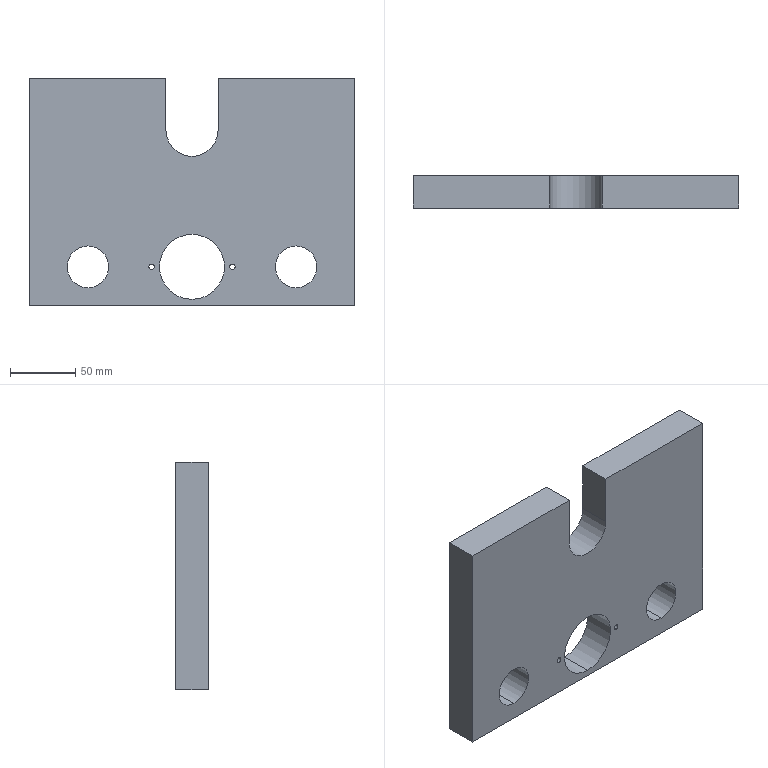Part | SolidWorks | features ICE 3, HoleWzd 2, Extrusion 1, MirrorPattern 1 | 1 solid | 52 faces | box 250 x 25 x 175 mm | volume 946629 mm3 | cylinder 27 | cone 16 | plane 9 | commonest cylinder face diameters 4.2 x20 32 x4 50 x2 40 x1
STEP:
#1=CARTESIAN_POINT('',(-31.,0.,-59.6));
#2=VERTEX_POINT('',#1);
#3=CARTESIAN_POINT('',(-31.,0.,-55.4));
#4=VERTEX_POINT('',#3);
#5=CARTESIAN_POINT('',(-31.,0.,-57.5));
#6=DIRECTION('',(0.,1.,0.));
#7=DIRECTION('',(0.,0.,1.));
#8=AXIS2_PLACEMENT_3D('',#5,#6,#7);
#9=CIRCLE('',#8,2.1);
#10=EDGE_CURVE('',#2,#4,#9,.T.);
#11=ORIENTED_EDGE('',*,*,#10,.F.);
#12=CARTESIAN_POINT('',(-31.,25.,-59.6));
#13=VERTEX_POINT('',#12);
#14=CARTESIAN_POINT('',(-31.,25.,-59.6));
#15=DIRECTION('',(0.,1.,0.));
#16=VECTOR('',#15,1000.);
#17=LINE('',#14,#16);
#18=EDGE_CURVE('',#2,#13,#17,.T.);
#19=ORIENTED_EDGE('',*,*,#18,.T.);
#20=CARTESIAN_POINT('',(-31.,25.,-55.4));
#21=VERTEX_POINT('',#20);
#22=CARTESIAN_POINT('',(-31.,25.,-57.5));
#23=DIRECTION('',(0.,1.,0.));
#24=DIRECTION('',(0.,0.,1.));
#25=AXIS2_PLACEMENT_3D('',#22,#23,#24);
#26=CIRCLE('',#25,2.1);
#27=EDGE_CURVE('',#13,#21,#26,.T.);
#28=ORIENTED_EDGE('',*,*,#27,.T.);
#29=CARTESIAN_POINT('',(-31.,25.,-55.4));
#30=DIRECTION('',(0.,1.,0.));
#31=VECTOR('',#30,1000.);
#32=LINE('',#29,#31);
#33=EDGE_CURVE('',#4,#21,#32,.T.);
#34=ORIENTED_EDGE('',*,*,#33,.F.);
#35=EDGE_LOOP('',(#11,#19,#28,#34));
#36=FACE_OUTER_BOUND('',#35,.T.);
#37=CARTESIAN_POINT('',(-31.,25.,-57.5));
#38=DIRECTION('',(0.,1.,0.));
#39=DIRECTION('',(0.,0.,1.));
#40=AXIS2_PLACEMENT_3D('',#37,#38,#39);
#41=CYLINDRICAL_SURFACE('',#40,2.1);
#42=ADVANCED_FACE('',(#36),#41,.F.);
#43=CARTESIAN_POINT('',(31.,0.,-59.6));
#44=VERTEX_POINT('',#43);
#45=CARTESIAN_POINT('',(31.,0.,-55.4));
#46=VERTEX_POINT('',#45);
#47=CARTESIAN_POINT('',(31.,0.,-57.5));
#48=DIRECTION('',(0.,1.,0.));
#49=DIRECTION('',(0.,0.,1.));
#50=AXIS2_PLACEMENT_3D('',#47,#48,#49);
#51=CIRCLE('',#50,2.1);
#52=EDGE_CURVE('',#44,#46,#51,.T.);
#53=ORIENTED_EDGE('',*,*,#52,.F.);
#54=CARTESIAN_POINT('',(31.,25.,-59.6));
#55=VERTEX_POINT('',#54);
#56=CARTESIAN_POINT('',(31.,25.,-59.6));
#57=DIRECTION('',(0.,1.,0.));
#58=VECTOR('',#57,1000.);
#59=LINE('',#56,#58);
#60=EDGE_CURVE('',#44,#55,#59,.T.);
#61=ORIENTED_EDGE('',*,*,#60,.T.);
#62=CARTESIAN_POINT('',(31.,25.,-55.4));
#63=VERTEX_POINT('',#62);
#64=CARTESIAN_POINT('',(31.,25.,-57.5));
#65=DIRECTION('',(0.,1.,0.));
#66=DIRECTION('',(0.,0.,1.));
#67=AXIS2_PLACEMENT_3D('',#64,#65,#66);
#68=CIRCLE('',#67,2.1);
#69=EDGE_CURVE('',#55,#63,#68,.T.);
#70=ORIENTED_EDGE('',*,*,#69,.T.);
#71=CARTESIAN_POINT('',(31.,25.,-55.4));
#72=DIRECTION('',(0.,1.,0.));
#73=VECTOR('',#72,1000.);
#74=LINE('',#71,#73);
#75=EDGE_CURVE('',#46,#63,#74,.T.);
#76=ORIENTED_EDGE('',*,*,#75,.F.);
#77=EDGE_LOOP('',(#53,#61,#70,#76));
#78=FACE_OUTER_BOUND('',#77,.T.);
#79=CARTESIAN_POINT('',(31.,25.,-57.5));
#80=DIRECTION('',(0.,1.,0.));
#81=DIRECTION('',(0.,0.,1.));
#82=AXIS2_PLACEMENT_3D('',#79,#80,#81);
#83=CYLINDRICAL_SURFACE('',#82,2.1);
#84=ADVANCED_FACE('',(#78),#83,.F.);
#85=CARTESIAN_POINT('',(0.,0.,-82.5));
#86=VERTEX_POINT('',#85);
#87=CARTESIAN_POINT('',(0.,0.,-32.5));
#88=VERTEX_POINT('',#87);
#89=CARTESIAN_POINT('',(0.,0.,-57.5));
#90=DIRECTION('',(0.,1.,0.));
#91=DIRECTION('',(0.,0.,1.));
#92=AXIS2_PLACEMENT_3D('',#89,#90,#91);
#93=CIRCLE('',#92,25.);
#94=EDGE_CURVE('',#86,#88,#93,.T.);
#95=ORIENTED_EDGE('',*,*,#94,.F.);
#96=CARTESIAN_POINT('',(0.,25.,-82.5));
#97=VERTEX_POINT('',#96);
#98=CARTESIAN_POINT('',(0.,0.,-82.5));
#99=DIRECTION('',(0.,1.,0.));
#100=VECTOR('',#99,1000.);
#101=LINE('',#98,#100);
#102=EDGE_CURVE('',#86,#97,#101,.T.);
#103=ORIENTED_EDGE('',*,*,#102,.T.);
#104=CARTESIAN_POINT('',(0.,25.,-32.5));
#105=VERTEX_POINT('',#104);
#106=CARTESIAN_POINT('',(0.,25.,-57.5));
#107=DIRECTION('',(0.,1.,0.));
#108=DIRECTION('',(0.,0.,1.));
#109=AXIS2_PLACEMENT_3D('',#106,#107,#108);
#110=CIRCLE('',#109,25.);
#111=EDGE_CURVE('',#97,#105,#110,.T.);
#112=ORIENTED_EDGE('',*,*,#111,.T.);
#113=CARTESIAN_POINT('',(0.,0.,-32.5));
#114=DIRECTION('',(0.,1.,0.));
#115=VECTOR('',#114,1000.);
#116=LINE('',#113,#115);
#117=EDGE_CURVE('',#88,#105,#116,.T.);
#118=ORIENTED_EDGE('',*,*,#117,.F.);
#119=EDGE_LOOP('',(#95,#103,#112,#118));
#120=FACE_OUTER_BOUND('',#119,.T.);
#121=CARTESIAN_POINT('',(0.,0.,-57.5));
#122=DIRECTION('',(0.,1.,0.));
#123=DIRECTION('',(0.,0.,1.));
#124=AXIS2_PLACEMENT_3D('',#121,#122,#123);
#125=CYLINDRICAL_SURFACE('',#124,25.);
#126=ADVANCED_FACE('',(#120),#125,.F.);
#127=CARTESIAN_POINT('',(92.,12.6,-77.6));
#128=VERTEX_POINT('',#127);
#129=CARTESIAN_POINT('',(92.,12.6,-73.4));
#130=VERTEX_POINT('',#129);
#131=CARTESIAN_POINT('',(92.,12.6,-75.5));
#132=DIRECTION('',(0.,1.,0.));
#133=DIRECTION('',(0.,0.,1.));
#134=AXIS2_PLACEMENT_3D('',#131,#132,#133);
#135=CIRCLE('',#134,2.1);
#136=EDGE_CURVE('',#128,#130,#135,.T.);
#137=ORIENTED_EDGE('',*,*,#136,.F.);
#138=CARTESIAN_POINT('',(92.,25.,-77.6));
#139=VERTEX_POINT('',#138);
#140=CARTESIAN_POINT('',(92.,25.,-77.6));
#141=DIRECTION('',(0.,1.,0.));
#142=VECTOR('',#141,1000.);
#143=LINE('',#140,#142);
#144=EDGE_CURVE('',#128,#139,#143,.T.);
#145=ORIENTED_EDGE('',*,*,#144,.T.);
#146=CARTESIAN_POINT('',(92.,25.,-73.4));
#147=VERTEX_POINT('',#146);
#148=CARTESIAN_POINT('',(92.,25.,-75.5));
#149=DIRECTION('',(0.,1.,0.));
#150=DIRECTION('',(0.,0.,1.));
#151=AXIS2_PLACEMENT_3D('',#148,#149,#150);
#152=CIRCLE('',#151,2.1);
#153=EDGE_CURVE('',#139,#147,#152,.T.);
#154=ORIENTED_EDGE('',*,*,#153,.T.);
#155=CARTESIAN_POINT('',(92.,25.,-73.4));
#156=DIRECTION('',(0.,1.,0.));
#157=VECTOR('',#156,1000.);
#158=LINE('',#155,#157);
#159=EDGE_CURVE('',#130,#147,#158,.T.);
#160=ORIENTED_EDGE('',*,*,#159,.F.);
#161=EDGE_LOOP('',(#137,#145,#154,#160));
#162=FACE_OUTER_BOUND('',#161,.T.);
#163=CARTESIAN_POINT('',(92.,25.,-75.5));
#164=DIRECTION('',(0.,1.,0.));
#165=DIRECTION('',(0.,0.,1.));
#166=AXIS2_PLACEMENT_3D('',#163,#164,#165);
#167=CYLINDRICAL_SURFACE('',#166,2.1);
#168=ADVANCED_FACE('',(#162),#167,.F.);
#169=CARTESIAN_POINT('',(92.,11.338,-75.5));
#170=VERTEX_POINT('',#169);
#171=CARTESIAN_POINT('',(92.,12.6,-73.4));
#172=DIRECTION('',(0.,0.515,0.8572));
#173=VECTOR('',#172,1000.);
#174=LINE('',#171,#173);
#175=EDGE_CURVE('',#170,#130,#174,.T.);
#176=ORIENTED_EDGE('',*,*,#175,.F.);
#177=CARTESIAN_POINT('',(92.,12.6,-77.6));
#178=DIRECTION('',(0.,0.515,-0.8572));
#179=VECTOR('',#178,1000.);
#180=LINE('',#177,#179);
#181=EDGE_CURVE('',#170,#128,#180,.T.);
#182=ORIENTED_EDGE('',*,*,#181,.T.);
#183=ORIENTED_EDGE('',*,*,#136,.T.);
#184=EDGE_LOOP('',(#176,#182,#183));
#185=FACE_OUTER_BOUND('',#184,.T.);
#186=CARTESIAN_POINT('',(92.,12.6,-75.5));
#187=DIRECTION('',(0.,1.,0.));
#188=DIRECTION('',(0.,0.,1.));
#189=AXIS2_PLACEMENT_3D('',#186,#187,#188);
#190=CONICAL_SURFACE('',#189,2.1,1.03);
#191=ADVANCED_FACE('',(#185),#190,.F.);
#192=CARTESIAN_POINT('',(68.,12.6,-77.6));
#193=VERTEX_POINT('',#192);
#194=CARTESIAN_POINT('',(68.,12.6,-73.4));
#195=VERTEX_POINT('',#194);
#196=CARTESIAN_POINT('',(68.,12.6,-75.5));
#197=DIRECTION('',(0.,1.,0.));
#198=DIRECTION('',(0.,0.,1.));
#199=AXIS2_PLACEMENT_3D('',#196,#197,#198);
#200=CIRCLE('',#199,2.1);
#201=EDGE_CURVE('',#193,#195,#200,.T.);
#202=ORIENTED_EDGE('',*,*,#201,.F.);
#203=CARTESIAN_POINT('',(68.,25.,-77.6));
#204=VERTEX_POINT('',#203);
#205=CARTESIAN_POINT('',(68.,25.,-77.6));
#206=DIRECTION('',(0.,1.,0.));
#207=VECTOR('',#206,1000.);
#208=LINE('',#205,#207);
#209=EDGE_CURVE('',#193,#204,#208,.T.);
#210=ORIENTED_EDGE('',*,*,#209,.T.);
#211=CARTESIAN_POINT('',(68.,25.,-73.4));
#212=VERTEX_POINT('',#211);
#213=CARTESIAN_POINT('',(68.,25.,-75.5));
#214=DIRECTION('',(0.,1.,0.));
#215=DIRECTION('',(0.,0.,1.));
#216=AXIS2_PLACEMENT_3D('',#213,#214,#215);
#217=CIRCLE('',#216,2.1);
#218=EDGE_CURVE('',#204,#212,#217,.T.);
#219=ORIENTED_EDGE('',*,*,#218,.T.);
#220=CARTESIAN_POINT('',(68.,25.,-73.4));
#221=DIRECTION('',(0.,1.,0.));
#222=VECTOR('',#221,1000.);
#223=LINE('',#220,#222);
#224=EDGE_CURVE('',#195,#212,#223,.T.);
#225=ORIENTED_EDGE('',*,*,#224,.F.);
#226=EDGE_LOOP('',(#202,#210,#219,#225));
#227=FACE_OUTER_BOUND('',#226,.T.);
#228=CARTESIAN_POINT('',(68.,25.,-75.5));
#229=DIRECTION('',(0.,1.,0.));
#230=DIRECTION('',(0.,0.,1.));
#231=AXIS2_PLACEMENT_3D('',#228,#229,#230);
#232=CYLINDRICAL_SURFACE('',#231,2.1);
#233=ADVANCED_FACE('',(#227),#232,.F.);
#234=CARTESIAN_POINT('',(68.,11.338,-75.5));
#235=VERTEX_POINT('',#234);
#236=CARTESIAN_POINT('',(68.,12.6,-73.4));
#237=DIRECTION('',(0.,0.515,0.8572));
#238=VECTOR('',#237,1000.);
#239=LINE('',#236,#238);
#240=EDGE_CURVE('',#235,#195,#239,.T.);
#241=ORIENTED_EDGE('',*,*,#240,.F.);
#242=CARTESIAN_POINT('',(68.,12.6,-77.6));
#243=DIRECTION('',(0.,0.515,-0.8572));
#244=VECTOR('',#243,1000.);
#245=LINE('',#242,#244);
#246=EDGE_CURVE('',#235,#193,#245,.T.);
#247=ORIENTED_EDGE('',*,*,#246,.T.);
#248=ORIENTED_EDGE('',*,*,#201,.T.);
#249=EDGE_LOOP('',(#241,#247,#248));
#250=FACE_OUTER_BOUND('',#249,.T.);
#251=CARTESIAN_POINT('',(68.,12.6,-75.5));
#252=DIRECTION('',(0.,1.,0.));
#253=DIRECTION('',(0.,0.,1.));
#254=AXIS2_PLACEMENT_3D('',#251,#252,#253);
#255=CONICAL_SURFACE('',#254,2.1,1.03);
#256=ADVANCED_FACE('',(#250),#255,.F.);
#257=CARTESIAN_POINT('',(92.,12.6,-41.6));
#258=VERTEX_POINT('',#257);
#259=CARTESIAN_POINT('',(92.,12.6,-37.4));
#260=VERTEX_POINT('',#259);
#261=CARTESIAN_POINT('',(92.,12.6,-39.5));
#262=DIRECTION('',(0.,1.,0.));
#263=DIRECTION('',(0.,0.,1.));
#264=AXIS2_PLACEMENT_3D('',#261,#262,#263);
#265=CIRCLE('',#264,2.1);
#266=EDGE_CURVE('',#258,#260,#265,.T.);
#267=ORIENTED_EDGE('',*,*,#266,.F.);
#268=CARTESIAN_POINT('',(92.,25.,-41.6));
#269=VERTEX_POINT('',#268);
#270=CARTESIAN_POINT('',(92.,25.,-41.6));
#271=DIRECTION('',(0.,1.,0.));
#272=VECTOR('',#271,1000.);
#273=LINE('',#270,#272);
#274=EDGE_CURVE('',#258,#269,#273,.T.);
#275=ORIENTED_EDGE('',*,*,#274,.T.);
#276=CARTESIAN_POINT('',(92.,25.,-37.4));
#277=VERTEX_POINT('',#276);
#278=CARTESIAN_POINT('',(92.,25.,-39.5));
#279=DIRECTION('',(0.,1.,0.));
#280=DIRECTION('',(0.,0.,1.));
#281=AXIS2_PLACEMENT_3D('',#278,#279,#280);
#282=CIRCLE('',#281,2.1);
#283=EDGE_CURVE('',#269,#277,#282,.T.);
#284=ORIENTED_EDGE('',*,*,#283,.T.);
#285=CARTESIAN_POINT('',(92.,25.,-37.4));
#286=DIRECTION('',(0.,1.,0.));
#287=VECTOR('',#286,1000.);
#288=LINE('',#285,#287);
#289=EDGE_CURVE('',#260,#277,#288,.T.);
#290=ORIENTED_EDGE('',*,*,#289,.F.);
#291=EDGE_LOOP('',(#267,#275,#284,#290));
#292=FACE_OUTER_BOUND('',#291,.T.);
#293=CARTESIAN_POINT('',(92.,25.,-39.5));
#294=DIRECTION('',(0.,1.,0.));
#295=DIRECTION('',(0.,0.,1.));
#296=AXIS2_PLACEMENT_3D('',#293,#294,#295);
#297=CYLINDRICAL_SURFACE('',#296,2.1);
#298=ADVANCED_FACE('',(#292),#297,.F.);
#299=CARTESIAN_POINT('',(92.,11.338,-39.5));
#300=VERTEX_POINT('',#299);
#301=CARTESIAN_POINT('',(92.,12.6,-37.4));
#302=DIRECTION('',(0.,0.515,0.8572));
#303=VECTOR('',#302,1000.);
#304=LINE('',#301,#303);
#305=EDGE_CURVE('',#300,#260,#304,.T.);
#306=ORIENTED_EDGE('',*,*,#305,.F.);
#307=CARTESIAN_POINT('',(92.,12.6,-41.6));
#308=DIRECTION('',(0.,0.515,-0.8572));
#309=VECTOR('',#308,1000.);
#310=LINE('',#307,#309);
#311=EDGE_CURVE('',#300,#258,#310,.T.);
#312=ORIENTED_EDGE('',*,*,#311,.T.);
#313=ORIENTED_EDGE('',*,*,#266,.T.);
#314=EDGE_LOOP('',(#306,#312,#313));
#315=FACE_OUTER_BOUND('',#314,.T.);
#316=CARTESIAN_POINT('',(92.,12.6,-39.5));
#317=DIRECTION('',(0.,1.,0.));
#318=DIRECTION('',(0.,0.,1.));
#319=AXIS2_PLACEMENT_3D('',#316,#317,#318);
#320=CONICAL_SURFACE('',#319,2.1,1.03);
#321=ADVANCED_FACE('',(#315),#320,.F.);
#322=CARTESIAN_POINT('',(68.,12.6,-41.6));
#323=VERTEX_POINT('',#322);
#324=CARTESIAN_POINT('',(68.,12.6,-37.4));
#325=VERTEX_POINT('',#324);
#326=CARTESIAN_POINT('',(68.,12.6,-39.5));
#327=DIRECTION('',(0.,1.,0.));
#328=DIRECTION('',(0.,0.,1.));
#329=AXIS2_PLACEMENT_3D('',#326,#327,#328);
#330=CIRCLE('',#329,2.1);
#331=EDGE_CURVE('',#323,#325,#330,.T.);
#332=ORIENTED_EDGE('',*,*,#331,.F.);
#333=CARTESIAN_POINT('',(68.,25.,-41.6));
#334=VERTEX_POINT('',#333);
#335=CARTESIAN_POINT('',(68.,25.,-41.6));
#336=DIRECTION('',(0.,1.,0.));
#337=VECTOR('',#336,1000.);
#338=LINE('',#335,#337);
#339=EDGE_CURVE('',#323,#334,#338,.T.);
#340=ORIENTED_EDGE('',*,*,#339,.T.);
#341=CARTESIAN_POINT('',(68.,25.,-37.4));
#342=VERTEX_POINT('',#341);
#343=CARTESIAN_POINT('',(68.,25.,-39.5));
#344=DIRECTION('',(0.,1.,0.));
#345=DIRECTION('',(0.,0.,1.));
#346=AXIS2_PLACEMENT_3D('',#343,#344,#345);
#347=CIRCLE('',#346,2.1);
#348=EDGE_CURVE('',#334,#342,#347,.T.);
#349=ORIENTED_EDGE('',*,*,#348,.T.);
#350=CARTESIAN_POINT('',(68.,25.,-37.4));
#351=DIRECTION('',(0.,1.,0.));
#352=VECTOR('',#351,1000.);
#353=LINE('',#350,#352);
#354=EDGE_CURVE('',#325,#342,#353,.T.);
#355=ORIENTED_EDGE('',*,*,#354,.F.);
#356=EDGE_LOOP('',(#332,#340,#349,#355));
#357=FACE_OUTER_BOUND('',#356,.T.);
#358=CARTESIAN_POINT('',(68.,25.,-39.5));
#359=DIRECTION('',(0.,1.,0.));
#360=DIRECTION('',(0.,0.,1.));
#361=AXIS2_PLACEMENT_3D('',#358,#359,#360);
#362=CYLINDRICAL_SURFACE('',#361,2.1);
#363=ADVANCED_FACE('',(#357),#362,.F.);
#364=CARTESIAN_POINT('',(68.,11.338,-39.5));
#365=VERTEX_POINT('',#364);
#366=CARTESIAN_POINT('',(68.,12.6,-37.4));
#367=DIRECTION('',(0.,0.515,0.8572));
#368=VECTOR('',#367,1000.);
#369=LINE('',#366,#368);
#370=EDGE_CURVE('',#365,#325,#369,.T.);
#371=ORIENTED_EDGE('',*,*,#370,.F.);
#372=CARTESIAN_POINT('',(68.,12.6,-41.6));
#373=DIRECTION('',(0.,0.515,-0.8572));
#374=VECTOR('',#373,1000.);
#375=LINE('',#372,#374);
#376=EDGE_CURVE('',#365,#323,#375,.T.);
#377=ORIENTED_EDGE('',*,*,#376,.T.);
#378=ORIENTED_EDGE('',*,*,#331,.T.);
#379=EDGE_LOOP('',(#371,#377,#378));
#380=FACE_OUTER_BOUND('',#379,.T.);
#381=CARTESIAN_POINT('',(68.,12.6,-39.5));
#382=DIRECTION('',(0.,1.,0.));
#383=DIRECTION('',(0.,0.,1.));
#384=AXIS2_PLACEMENT_3D('',#381,#382,#383);
#385=CONICAL_SURFACE('',#384,2.1,1.03);
#386=ADVANCED_FACE('',(#380),#385,.F.);
#387=CARTESIAN_POINT('',(-92.,12.6,-77.6));
#388=VERTEX_POINT('',#387);
#389=CARTESIAN_POINT('',(-92.,12.6,-73.4));
#390=VERTEX_POINT('',#389);
#391=CARTESIAN_POINT('',(-92.,12.6,-75.5));
#392=DIRECTION('',(0.,1.,0.));
#393=DIRECTION('',(0.,0.,1.));
#394=AXIS2_PLACEMENT_3D('',#391,#392,#393);
#395=CIRCLE('',#394,2.1);
#396=EDGE_CURVE('',#388,#390,#395,.T.);
#397=ORIENTED_EDGE('',*,*,#396,.F.);
#398=CARTESIAN_POINT('',(-92.,25.,-77.6));
#399=VERTEX_POINT('',#398);
#400=CARTESIAN_POINT('',(-92.,25.,-77.6));
#401=DIRECTION('',(0.,1.,0.));
#402=VECTOR('',#401,1000.);
#403=LINE('',#400,#402);
#404=EDGE_CURVE('',#388,#399,#403,.T.);
#405=ORIENTED_EDGE('',*,*,#404,.T.);
#406=CARTESIAN_POINT('',(-92.,25.,-73.4));
#407=VERTEX_POINT('',#406);
#408=CARTESIAN_POINT('',(-92.,25.,-75.5));
#409=DIRECTION('',(0.,1.,0.));
#410=DIRECTION('',(0.,0.,1.));
#411=AXIS2_PLACEMENT_3D('',#408,#409,#410);
#412=CIRCLE('',#411,2.1);
#413=EDGE_CURVE('',#399,#407,#412,.T.);
#414=ORIENTED_EDGE('',*,*,#413,.T.);
#415=CARTESIAN_POINT('',(-92.,25.,-73.4));
#416=DIRECTION('',(0.,1.,0.));
#417=VECTOR('',#416,1000.);
#418=LINE('',#415,#417);
#419=EDGE_CURVE('',#390,#407,#418,.T.);
#420=ORIENTED_EDGE('',*,*,#419,.F.);
#421=EDGE_LOOP('',(#397,#405,#414,#420));
#422=FACE_OUTER_BOUND('',#421,.T.);
#423=CARTESIAN_POINT('',(-92.,25.,-75.5));
#424=DIRECTION('',(0.,1.,0.));
#425=DIRECTION('',(0.,0.,1.));
#426=AXIS2_PLACEMENT_3D('',#423,#424,#425);
#427=CYLINDRICAL_SURFACE('',#426,2.1);
#428=ADVANCED_FACE('',(#422),#427,.F.);
#429=CARTESIAN_POINT('',(-92.,11.338,-75.5));
#430=VERTEX_POINT('',#429);
#431=CARTESIAN_POINT('',(-92.,12.6,-73.4));
#432=DIRECTION('',(0.,0.515,0.8572));
#433=VECTOR('',#432,1000.);
#434=LINE('',#431,#433);
#435=EDGE_CURVE('',#430,#390,#434,.T.);
#436=ORIENTED_EDGE('',*,*,#435,.F.);
#437=CARTESIAN_POINT('',(-92.,12.6,-77.6));
#438=DIRECTION('',(0.,0.515,-0.8572));
#439=VECTOR('',#438,1000.);
#440=LINE('',#437,#439);
#441=EDGE_CURVE('',#430,#388,#440,.T.);
#442=ORIENTED_EDGE('',*,*,#441,.T.);
#443=ORIENTED_EDGE('',*,*,#396,.T.);
#444=EDGE_LOOP('',(#436,#442,#443));
#445=FACE_OUTER_BOUND('',#444,.T.);
#446=CARTESIAN_POINT('',(-92.,12.6,-75.5));
#447=DIRECTION('',(0.,1.,0.));
#448=DIRECTION('',(0.,0.,1.));
#449=AXIS2_PLACEMENT_3D('',#446,#447,#448);
#450=CONICAL_SURFACE('',#449,2.1,1.03);
#451=ADVANCED_FACE('',(#445),#450,.F.);
#452=CARTESIAN_POINT('',(-68.,12.6,-77.6));
#453=VERTEX_POINT('',#452);
#454=CARTESIAN_POINT('',(-68.,12.6,-73.4));
#455=VERTEX_POINT('',#454);
#456=CARTESIAN_POINT('',(-68.,12.6,-75.5));
#457=DIRECTION('',(0.,1.,0.));
#458=DIRECTION('',(0.,0.,1.));
#459=AXIS2_PLACEMENT_3D('',#456,#457,#458);
#460=CIRCLE('',#459,2.1);
#461=EDGE_CURVE('',#453,#455,#460,.T.);
#462=ORIENTED_EDGE('',*,*,#461,.F.);
#463=CARTESIAN_POINT('',(-68.,25.,-77.6));
#464=VERTEX_POINT('',#463);
#465=CARTESIAN_POINT('',(-68.,25.,-77.6));
#466=DIRECTION('',(0.,1.,0.));
#467=VECTOR('',#466,1000.);
#468=LINE('',#465,#467);
#469=EDGE_CURVE('',#453,#464,#468,.T.);
#470=ORIENTED_EDGE('',*,*,#469,.T.);
#471=CARTESIAN_POINT('',(-68.,25.,-73.4));
#472=VERTEX_POINT('',#471);
#473=CARTESIAN_POINT('',(-68.,25.,-75.5));
#474=DIRECTION('',(0.,1.,0.));
#475=DIRECTION('',(0.,0.,1.));
#476=AXIS2_PLACEMENT_3D('',#473,#474,#475);
#477=CIRCLE('',#476,2.1);
#478=EDGE_CURVE('',#464,#472,#477,.T.);
#479=ORIENTED_EDGE('',*,*,#478,.T.);
#480=CARTESIAN_POINT('',(-68.,25.,-73.4));
#481=DIRECTION('',(0.,1.,0.));
#482=VECTOR('',#481,1000.);
#483=LINE('',#480,#482);
#484=EDGE_CURVE('',#455,#472,#483,.T.);
#485=ORIENTED_EDGE('',*,*,#484,.F.);
#486=EDGE_LOOP('',(#462,#470,#479,#485));
#487=FACE_OUTER_BOUND('',#486,.T.);
#488=CARTESIAN_POINT('',(-68.,25.,-75.5));
#489=DIRECTION('',(0.,1.,0.));
#490=DIRECTION('',(0.,0.,1.));
#491=AXIS2_PLACEMENT_3D('',#488,#489,#490);
#492=CYLINDRICAL_SURFACE('',#491,2.1);
#493=ADVANCED_FACE('',(#487),#492,.F.);
#494=CARTESIAN_POINT('',(-68.,11.338,-75.5));
#495=VERTEX_POINT('',#494);
#496=CARTESIAN_POINT('',(-68.,12.6,-73.4));
#497=DIRECTION('',(0.,0.515,0.8572));
#498=VECTOR('',#497,1000.);
#499=LINE('',#496,#498);
#500=EDGE_CURVE('',#495,#455,#499,.T.);
#501=ORIENTED_EDGE('',*,*,#500,.F.);
#502=CARTESIAN_POINT('',(-68.,12.6,-77.6));
#503=DIRECTION('',(0.,0.515,-0.8572));
#504=VECTOR('',#503,1000.);
#505=LINE('',#502,#504);
#506=EDGE_CURVE('',#495,#453,#505,.T.);
#507=ORIENTED_EDGE('',*,*,#506,.T.);
#508=ORIENTED_EDGE('',*,*,#461,.T.);
#509=EDGE_LOOP('',(#501,#507,#508));
#510=FACE_OUTER_BOUND('',#509,.T.);
#511=CARTESIAN_POINT('',(-68.,12.6,-75.5));
#512=DIRECTION('',(0.,1.,0.));
#513=DIRECTION('',(0.,0.,1.));
#514=AXIS2_PLACEMENT_3D('',#511,#512,#513);
#515=CONICAL_SURFACE('',#514,2.1,1.03);
#516=ADVANCED_FACE('',(#510),#515,.F.);
#517=CARTESIAN_POINT('',(-92.,12.6,-41.6));
#518=VERTEX_POINT('',#517);
#519=CARTESIAN_POINT('',(-92.,12.6,-37.4));
#520=VERTEX_POINT('',#519);
#521=CARTESIAN_POINT('',(-92.,12.6,-39.5));
#522=DIRECTION('',(0.,1.,0.));
#523=DIRECTION('',(0.,0.,1.));
#524=AXIS2_PLACEMENT_3D('',#521,#522,#523);
#525=CIRCLE('',#524,2.1);
#526=EDGE_CURVE('',#518,#520,#525,.T.);
#527=ORIENTED_EDGE('',*,*,#526,.F.);
#528=CARTESIAN_POINT('',(-92.,25.,-41.6));
#529=VERTEX_POINT('',#528);
#530=CARTESIAN_POINT('',(-92.,25.,-41.6));
#531=DIRECTION('',(0.,1.,0.));
#532=VECTOR('',#531,1000.);
#533=LINE('',#530,#532);
#534=EDGE_CURVE('',#518,#529,#533,.T.);
#535=ORIENTED_EDGE('',*,*,#534,.T.);
#536=CARTESIAN_POINT('',(-92.,25.,-37.4));
#537=VERTEX_POINT('',#536);
#538=CARTESIAN_POINT('',(-92.,25.,-39.5));
#539=DIRECTION('',(0.,1.,0.));
#540=DIRECTION('',(0.,0.,1.));
#541=AXIS2_PLACEMENT_3D('',#538,#539,#540);
#542=CIRCLE('',#541,2.1);
#543=EDGE_CURVE('',#529,#537,#542,.T.);
#544=ORIENTED_EDGE('',*,*,#543,.T.);
#545=CARTESIAN_POINT('',(-92.,25.,-37.4));
#546=DIRECTION('',(0.,1.,0.));
#547=VECTOR('',#546,1000.);
#548=LINE('',#545,#547);
#549=EDGE_CURVE('',#520,#537,#548,.T.);
#550=ORIENTED_EDGE('',*,*,#549,.F.);
#551=EDGE_LOOP('',(#527,#535,#544,#550));
#552=FACE_OUTER_BOUND('',#551,.T.);
#553=CARTESIAN_POINT('',(-92.,25.,-39.5));
#554=DIRECTION('',(0.,1.,0.));
#555=DIRECTION('',(0.,0.,1.));
#556=AXIS2_PLACEMENT_3D('',#553,#554,#555);
#557=CYLINDRICAL_SURFACE('',#556,2.1);
#558=ADVANCED_FACE('',(#552),#557,.F.);
#559=CARTESIAN_POINT('',(-92.,11.338,-39.5));
#560=VERTEX_POINT('',#559);
#561=CARTESIAN_POINT('',(-92.,12.6,-37.4));
#562=DIRECTION('',(0.,0.515,0.8572));
#563=VECTOR('',#562,1000.);
#564=LINE('',#561,#563);
#565=EDGE_CURVE('',#560,#520,#564,.T.);
#566=ORIENTED_EDGE('',*,*,#565,.F.);
#567=CARTESIAN_POINT('',(-92.,12.6,-41.6));
#568=DIRECTION('',(0.,0.515,-0.8572));
#569=VECTOR('',#568,1000.);
#570=LINE('',#567,#569);
#571=EDGE_CURVE('',#560,#518,#570,.T.);
#572=ORIENTED_EDGE('',*,*,#571,.T.);
#573=ORIENTED_EDGE('',*,*,#526,.T.);
#574=EDGE_LOOP('',(#566,#572,#573));
#575=FACE_OUTER_BOUND('',#574,.T.);
#576=CARTESIAN_POINT('',(-92.,12.6,-39.5));
#577=DIRECTION('',(0.,1.,0.));
#578=DIRECTION('',(0.,0.,1.));
#579=AXIS2_PLACEMENT_3D('',#576,#577,#578);
#580=CONICAL_SURFACE('',#579,2.1,1.03);
#581=ADVANCED_FACE('',(#575),#580,.F.);
#582=CARTESIAN_POINT('',(-68.,12.6,-41.6));
#583=VERTEX_POINT('',#582);
#584=CARTESIAN_POINT('',(-68.,12.6,-37.4));
#585=VERTEX_POINT('',#584);
#586=CARTESIAN_POINT('',(-68.,12.6,-39.5));
#587=DIRECTION('',(0.,1.,0.));
#588=DIRECTION('',(0.,0.,1.));
#589=AXIS2_PLACEMENT_3D('',#586,#587,#588);
#590=CIRCLE('',#589,2.1);
#591=EDGE_CURVE('',#583,#585,#590,.T.);
#592=ORIENTED_EDGE('',*,*,#591,.F.);
#593=CARTESIAN_POINT('',(-68.,25.,-41.6));
#594=VERTEX_POINT('',#593);
#595=CARTESIAN_POINT('',(-68.,25.,-41.6));
#596=DIRECTION('',(0.,1.,0.));
#597=VECTOR('',#596,1000.);
#598=LINE('',#595,#597);
#599=EDGE_CURVE('',#583,#594,#598,.T.);
#600=ORIENTED_EDGE('',*,*,#599,.T.);
#601=CARTESIAN_POINT('',(-68.,25.,-37.4));
#602=VERTEX_POINT('',#601);
#603=CARTESIAN_POINT('',(-68.,25.,-39.5));
#604=DIRECTION('',(0.,1.,0.));
#605=DIRECTION('',(0.,0.,1.));
#606=AXIS2_PLACEMENT_3D('',#603,#604,#605);
#607=CIRCLE('',#606,2.1);
#608=EDGE_CURVE('',#594,#602,#607,.T.);
#609=ORIENTED_EDGE('',*,*,#608,.T.);
#610=CARTESIAN_POINT('',(-68.,25.,-37.4));
#611=DIRECTION('',(0.,1.,0.));
#612=VECTOR('',#611,1000.);
#613=LINE('',#610,#612);
#614=EDGE_CURVE('',#585,#602,#613,.T.);
#615=ORIENTED_EDGE('',*,*,#614,.F.);
#616=EDGE_LOOP('',(#592,#600,#609,#615));
#617=FACE_OUTER_BOUND('',#616,.T.);
#618=CARTESIAN_POINT('',(-68.,25.,-39.5));
#619=DIRECTION('',(0.,1.,0.));
#620=DIRECTION('',(0.,0.,1.));
#621=AXIS2_PLACEMENT_3D('',#618,#619,#620);
#622=CYLINDRICAL_SURFACE('',#621,2.1);
#623=ADVANCED_FACE('',(#617),#622,.F.);
#624=CARTESIAN_POINT('',(-68.,11.338,-39.5));
#625=VERTEX_POINT('',#624);
#626=CARTESIAN_POINT('',(-68.,12.6,-37.4));
#627=DIRECTION('',(0.,0.515,0.8572));
#628=VECTOR('',#627,1000.);
#629=LINE('',#626,#628);
#630=EDGE_CURVE('',#625,#585,#629,.T.);
#631=ORIENTED_EDGE('',*,*,#630,.F.);
#632=CARTESIAN_POINT('',(-68.,12.6,-41.6));
#633=DIRECTION('',(0.,0.515,-0.8572));
#634=VECTOR('',#633,1000.);
#635=LINE('',#632,#634);
#636=EDGE_CURVE('',#625,#583,#635,.T.);
#637=ORIENTED_EDGE('',*,*,#636,.T.);
#638=ORIENTED_EDGE('',*,*,#591,.T.);
#639=EDGE_LOOP('',(#631,#637,#638));
#640=FACE_OUTER_BOUND('',#639,.T.);
#641=CARTESIAN_POINT('',(-68.,12.6,-39.5));
#642=DIRECTION('',(0.,1.,0.));
#643=DIRECTION('',(0.,0.,1.));
#644=AXIS2_PLACEMENT_3D('',#641,#642,#643);
#645=CONICAL_SURFACE('',#644,2.1,1.03);
#646=ADVANCED_FACE('',(#640),#645,.F.);
#647=CARTESIAN_POINT('',(-80.,0.,-73.5));
#648=VERTEX_POINT('',#647);
#649=CARTESIAN_POINT('',(-80.,0.,-41.5));
#650=VERTEX_POINT('',#649);
#651=CARTESIAN_POINT('',(-80.,0.,-57.5));
#652=DIRECTION('',(0.,1.,0.));
#653=DIRECTION('',(0.,0.,1.));
#654=AXIS2_PLACEMENT_3D('',#651,#652,#653);
#655=CIRCLE('',#654,16.);
#656=EDGE_CURVE('',#648,#650,#655,.T.);
#657=ORIENTED_EDGE('',*,*,#656,.F.);
#658=CARTESIAN_POINT('',(-80.,25.,-73.5));
#659=VERTEX_POINT('',#658);
#660=CARTESIAN_POINT('',(-80.,0.,-73.5));
#661=DIRECTION('',(0.,1.,0.));
#662=VECTOR('',#661,1000.);
#663=LINE('',#660,#662);
#664=EDGE_CURVE('',#648,#659,#663,.T.);
#665=ORIENTED_EDGE('',*,*,#664,.T.);
#666=CARTESIAN_POINT('',(-80.,25.,-41.5));
#667=VERTEX_POINT('',#666);
#668=CARTESIAN_POINT('',(-80.,25.,-57.5));
#669=DIRECTION('',(0.,1.,0.));
#670=DIRECTION('',(0.,0.,1.));
#671=AXIS2_PLACEMENT_3D('',#668,#669,#670);
#672=CIRCLE('',#671,16.);
#673=EDGE_CURVE('',#659,#667,#672,.T.);
#674=ORIENTED_EDGE('',*,*,#673,.T.);
#675=CARTESIAN_POINT('',(-80.,0.,-41.5));
#676=DIRECTION('',(0.,1.,0.));
#677=VECTOR('',#676,1000.);
#678=LINE('',#675,#677);
#679=EDGE_CURVE('',#650,#667,#678,.T.);
#680=ORIENTED_EDGE('',*,*,#679,.F.);
#681=EDGE_LOOP('',(#657,#665,#674,#680));
#682=FACE_OUTER_BOUND('',#681,.T.);
#683=CARTESIAN_POINT('',(-80.,0.,-57.5));
#684=DIRECTION('',(0.,1.,0.));
#685=DIRECTION('',(0.,0.,1.));
#686=AXIS2_PLACEMENT_3D('',#683,#684,#685);
#687=CYLINDRICAL_SURFACE('',#686,16.);
#688=ADVANCED_FACE('',(#682),#687,.F.);
#689=CARTESIAN_POINT('',(80.,0.,-73.5));
#690=VERTEX_POINT('',#689);
#691=CARTESIAN_POINT('',(80.,0.,-41.5));
#692=VERTEX_POINT('',#691);
#693=CARTESIAN_POINT('',(80.,0.,-57.5));
#694=DIRECTION('',(0.,1.,0.));
#695=DIRECTION('',(0.,0.,-1.));
#696=AXIS2_PLACEMENT_3D('',#693,#694,#695);
#697=CIRCLE('',#696,16.);
#698=EDGE_CURVE('',#690,#692,#697,.T.);
#699=ORIENTED_EDGE('',*,*,#698,.F.);
#700=CARTESIAN_POINT('',(80.,25.,-73.5));
#701=VERTEX_POINT('',#700);
#702=CARTESIAN_POINT('',(80.,0.,-73.5));
#703=DIRECTION('',(0.,1.,0.));
#704=VECTOR('',#703,1000.);
#705=LINE('',#702,#704);
#706=EDGE_CURVE('',#690,#701,#705,.T.);
#707=ORIENTED_EDGE('',*,*,#706,.T.);
#708=CARTESIAN_POINT('',(80.,25.,-41.5));
#709=VERTEX_POINT('',#708);
#710=CARTESIAN_POINT('',(80.,25.,-57.5));
#711=DIRECTION('',(0.,1.,0.));
#712=DIRECTION('',(0.,0.,-1.));
#713=AXIS2_PLACEMENT_3D('',#710,#711,#712);
#714=CIRCLE('',#713,16.);
#715=EDGE_CURVE('',#701,#709,#714,.T.);
#716=ORIENTED_EDGE('',*,*,#715,.T.);
#717=CARTESIAN_POINT('',(80.,0.,-41.5));
#718=DIRECTION('',(0.,1.,0.));
#719=VECTOR('',#718,1000.);
#720=LINE('',#717,#719);
#721=EDGE_CURVE('',#692,#709,#720,.T.);
#722=ORIENTED_EDGE('',*,*,#721,.F.);
#723=EDGE_LOOP('',(#699,#707,#716,#722));
#724=FACE_OUTER_BOUND('',#723,.T.);
#725=CARTESIAN_POINT('',(80.,0.,-57.5));
#726=DIRECTION('',(0.,1.,0.));
#727=DIRECTION('',(0.,0.,1.));
#728=AXIS2_PLACEMENT_3D('',#725,#726,#727);
#729=CYLINDRICAL_SURFACE('',#728,16.);
#730=ADVANCED_FACE('',(#724),#729,.F.);
#731=CARTESIAN_POINT('',(20.,25.,87.5));
#732=VERTEX_POINT('',#731);
#733=CARTESIAN_POINT('',(125.,25.,87.5));
#734=VERTEX_POINT('',#733);
#735=CARTESIAN_POINT('',(-125.,25.,87.5));
#736=DIRECTION('',(1.,0.,0.));
#737=VECTOR('',#736,1000.);
#738=LINE('',#735,#737);
#739=EDGE_CURVE('',#732,#734,#738,.T.);
#740=ORIENTED_EDGE('',*,*,#739,.F.);
#741=CARTESIAN_POINT('',(20.,0.,87.5));
#742=VERTEX_POINT('',#741);
#743=CARTESIAN_POINT('',(20.,0.,87.5));
#744=DIRECTION('',(0.,1.,0.));
#745=VECTOR('',#744,1000.);
#746=LINE('',#743,#745);
#747=EDGE_CURVE('',#742,#732,#746,.T.);
#748=ORIENTED_EDGE('',*,*,#747,.F.);
#749=CARTESIAN_POINT('',(125.,0.,87.5));
#750=VERTEX_POINT('',#749);
#751=CARTESIAN_POINT('',(-125.,0.,87.5));
#752=DIRECTION('',(1.,0.,0.));
#753=VECTOR('',#752,1000.);
#754=LINE('',#751,#753);
#755=EDGE_CURVE('',#742,#750,#754,.T.);
#756=ORIENTED_EDGE('',*,*,#755,.T.);
#757=CARTESIAN_POINT('',(125.,25.,87.5));
#758=DIRECTION('',(0.,-1.,0.));
#759=VECTOR('',#758,1000.);
#760=LINE('',#757,#759);
#761=EDGE_CURVE('',#734,#750,#760,.T.);
#762=ORIENTED_EDGE('',*,*,#761,.F.);
#763=EDGE_LOOP('',(#740,#748,#756,#762));
#764=FACE_OUTER_BOUND('',#763,.T.);
#765=CARTESIAN_POINT('',(-125.,25.,87.5));
#766=DIRECTION('',(0.,0.,-1.));
#767=DIRECTION('',(-1.,0.,0.));
#768=AXIS2_PLACEMENT_3D('',#765,#766,#767);
#769=PLANE('',#768);
#770=ADVANCED_FACE('',(#764),#769,.F.);
#771=CARTESIAN_POINT('',(125.,0.,-87.5));
#772=VERTEX_POINT('',#771);
#773=CARTESIAN_POINT('',(125.,0.,-87.5));
#774=DIRECTION('',(0.,0.,-1.));
#775=VECTOR('',#774,1000.);
#776=LINE('',#773,#775);
#777=EDGE_CURVE('',#750,#772,#776,.T.);
#778=ORIENTED_EDGE('',*,*,#777,.T.);
#779=CARTESIAN_POINT('',(125.,25.,-87.5));
#780=VERTEX_POINT('',#779);
#781=CARTESIAN_POINT('',(125.,25.,-87.5));
#782=DIRECTION('',(0.,-1.,0.));
#783=VECTOR('',#782,1000.);
#784=LINE('',#781,#783);
#785=EDGE_CURVE('',#780,#772,#784,.T.);
#786=ORIENTED_EDGE('',*,*,#785,.F.);
#787=CARTESIAN_POINT('',(125.,25.,-87.5));
#788=DIRECTION('',(0.,0.,-1.));
#789=VECTOR('',#788,1000.);
#790=LINE('',#787,#789);
#791=EDGE_CURVE('',#734,#780,#790,.T.);
#792=ORIENTED_EDGE('',*,*,#791,.F.);
#793=ORIENTED_EDGE('',*,*,#761,.T.);
#794=EDGE_LOOP('',(#778,#786,#792,#793));
#795=FACE_OUTER_BOUND('',#794,.T.);
#796=CARTESIAN_POINT('',(125.,25.,-87.5));
#797=DIRECTION('',(-1.,0.,0.));
#798=DIRECTION('',(0.,0.,1.));
#799=AXIS2_PLACEMENT_3D('',#796,#797,#798);
#800=PLANE('',#799);
#801=ADVANCED_FACE('',(#795),#800,.F.);
#802=CARTESIAN_POINT('',(-125.,0.,-87.5));
#803=VERTEX_POINT('',#802);
#804=CARTESIAN_POINT('',(-125.,0.,-87.5));
#805=DIRECTION('',(-1.,0.,0.));
#806=VECTOR('',#805,1000.);
#807=LINE('',#804,#806);
#808=EDGE_CURVE('',#772,#803,#807,.T.);
#809=ORIENTED_EDGE('',*,*,#808,.T.);
#810=CARTESIAN_POINT('',(-125.,25.,-87.5));
#811=VERTEX_POINT('',#810);
#812=CARTESIAN_POINT('',(-125.,25.,-87.5));
#813=DIRECTION('',(0.,-1.,0.));
#814=VECTOR('',#813,1000.);
#815=LINE('',#812,#814);
#816=EDGE_CURVE('',#811,#803,#815,.T.);
#817=ORIENTED_EDGE('',*,*,#816,.F.);
#818=CARTESIAN_POINT('',(-125.,25.,-87.5));
#819=DIRECTION('',(-1.,0.,0.));
#820=VECTOR('',#819,1000.);
#821=LINE('',#818,#820);
#822=EDGE_CURVE('',#780,#811,#821,.T.);
#823=ORIENTED_EDGE('',*,*,#822,.F.);
#824=ORIENTED_EDGE('',*,*,#785,.T.);
#825=EDGE_LOOP('',(#809,#817,#823,#824));
#826=FACE_OUTER_BOUND('',#825,.T.);
#827=CARTESIAN_POINT('',(-125.,25.,-87.5));
#828=DIRECTION('',(0.,0.,1.));
#829=DIRECTION('',(1.,0.,0.));
#830=AXIS2_PLACEMENT_3D('',#827,#828,#829);
#831=PLANE('',#830);
#832=ADVANCED_FACE('',(#826),#831,.F.);
#833=CARTESIAN_POINT('',(-125.,0.,87.5));
#834=VERTEX_POINT('',#833);
#835=CARTESIAN_POINT('',(-125.,0.,-87.5));
#836=DIRECTION('',(0.,0.,1.));
#837=VECTOR('',#836,1000.);
#838=LINE('',#835,#837);
#839=EDGE_CURVE('',#803,#834,#838,.T.);
#840=ORIENTED_EDGE('',*,*,#839,.T.);
#841=CARTESIAN_POINT('',(-125.,25.,87.5));
#842=VERTEX_POINT('',#841);
#843=CARTESIAN_POINT('',(-125.,25.,87.5));
#844=DIRECTION('',(0.,-1.,0.));
#845=VECTOR('',#844,1000.);
#846=LINE('',#843,#845);
#847=EDGE_CURVE('',#842,#834,#846,.T.);
#848=ORIENTED_EDGE('',*,*,#847,.F.);
#849=CARTESIAN_POINT('',(-125.,25.,-87.5));
#850=DIRECTION('',(0.,0.,1.));
#851=VECTOR('',#850,1000.);
#852=LINE('',#849,#851);
#853=EDGE_CURVE('',#811,#842,#852,.T.);
#854=ORIENTED_EDGE('',*,*,#853,.F.);
#855=ORIENTED_EDGE('',*,*,#816,.T.);
#856=EDGE_LOOP('',(#840,#848,#854,#855));
#857=FACE_OUTER_BOUND('',#856,.T.);
#858=CARTESIAN_POINT('',(-125.,25.,-87.5));
#859=DIRECTION('',(1.,0.,0.));
#860=DIRECTION('',(0.,0.,-1.));
#861=AXIS2_PLACEMENT_3D('',#858,#859,#860);
#862=PLANE('',#861);
#863=ADVANCED_FACE('',(#857),#862,.F.);
#864=CARTESIAN_POINT('',(-20.,0.,87.5));
#865=VERTEX_POINT('',#864);
#866=CARTESIAN_POINT('',(-125.,0.,87.5));
#867=DIRECTION('',(1.,0.,0.));
#868=VECTOR('',#867,1000.);
#869=LINE('',#866,#868);
#870=EDGE_CURVE('',#834,#865,#869,.T.);
#871=ORIENTED_EDGE('',*,*,#870,.T.);
#872=CARTESIAN_POINT('',(-20.,25.,87.5));
#873=VERTEX_POINT('',#872);
#874=CARTESIAN_POINT('',(-20.,0.,87.5));
#875=DIRECTION('',(0.,1.,0.));
#876=VECTOR('',#875,1000.);
#877=LINE('',#874,#876);
#878=EDGE_CURVE('',#865,#873,#877,.T.);
#879=ORIENTED_EDGE('',*,*,#878,.T.);
#880=CARTESIAN_POINT('',(-125.,25.,87.5));
#881=DIRECTION('',(1.,0.,0.));
#882=VECTOR('',#881,1000.);
#883=LINE('',#880,#882);
#884=EDGE_CURVE('',#842,#873,#883,.T.);
#885=ORIENTED_EDGE('',*,*,#884,.F.);
#886=ORIENTED_EDGE('',*,*,#847,.T.);
#887=EDGE_LOOP('',(#871,#879,#885,#886));
#888=FACE_OUTER_BOUND('',#887,.T.);
#889=CARTESIAN_POINT('',(-125.,25.,87.5));
#890=DIRECTION('',(0.,0.,-1.));
#891=DIRECTION('',(-1.,0.,0.));
#892=AXIS2_PLACEMENT_3D('',#889,#890,#891);
#893=PLANE('',#892);
#894=ADVANCED_FACE('',(#888),#893,.F.);
#895=CARTESIAN_POINT('',(-31.,25.,-57.5));
#896=DIRECTION('',(0.,1.,0.));
#897=DIRECTION('',(0.,0.,1.));
#898=AXIS2_PLACEMENT_3D('',#895,#896,#897);
#899=CIRCLE('',#898,2.1);
#900=EDGE_CURVE('',#21,#13,#899,.T.);
#901=ORIENTED_EDGE('',*,*,#900,.F.);
#902=ORIENTED_EDGE('',*,*,#27,.F.);
#903=EDGE_LOOP('',(#901,#902));
#904=FACE_BOUND('',#903,.T.);
#905=CARTESIAN_POINT('',(31.,25.,-57.5));
#906=DIRECTION('',(0.,1.,0.));
#907=DIRECTION('',(0.,0.,1.));
#908=AXIS2_PLACEMENT_3D('',#905,#906,#907);
#909=CIRCLE('',#908,2.1);
#910=EDGE_CURVE('',#63,#55,#909,.T.);
#911=ORIENTED_EDGE('',*,*,#910,.F.);
#912=ORIENTED_EDGE('',*,*,#69,.F.);
#913=EDGE_LOOP('',(#911,#912));
#914=FACE_BOUND('',#913,.T.);
#915=CARTESIAN_POINT('',(0.,25.,-57.5));
#916=DIRECTION('',(0.,1.,0.));
#917=DIRECTION('',(0.,0.,1.));
#918=AXIS2_PLACEMENT_3D('',#915,#916,#917);
#919=CIRCLE('',#918,25.);
#920=EDGE_CURVE('',#105,#97,#919,.T.);
#921=ORIENTED_EDGE('',*,*,#920,.F.);
#922=ORIENTED_EDGE('',*,*,#111,.F.);
#923=EDGE_LOOP('',(#921,#922));
#924=FACE_BOUND('',#923,.T.);
#925=CARTESIAN_POINT('',(92.,25.,-75.5));
#926=DIRECTION('',(0.,1.,0.));
#927=DIRECTION('',(0.,0.,1.));
#928=AXIS2_PLACEMENT_3D('',#925,#926,#927);
#929=CIRCLE('',#928,2.1);
#930=EDGE_CURVE('',#147,#139,#929,.T.);
#931=ORIENTED_EDGE('',*,*,#930,.F.);
#932=ORIENTED_EDGE('',*,*,#153,.F.);
#933=EDGE_LOOP('',(#931,#932));
#934=FACE_BOUND('',#933,.T.);
#935=CARTESIAN_POINT('',(68.,25.,-75.5));
#936=DIRECTION('',(0.,1.,0.));
#937=DIRECTION('',(0.,0.,1.));
#938=AXIS2_PLACEMENT_3D('',#935,#936,#937);
#939=CIRCLE('',#938,2.1);
#940=EDGE_CURVE('',#212,#204,#939,.T.);
#941=ORIENTED_EDGE('',*,*,#940,.F.);
#942=ORIENTED_EDGE('',*,*,#218,.F.);
#943=EDGE_LOOP('',(#941,#942));
#944=FACE_BOUND('',#943,.T.);
#945=CARTESIAN_POINT('',(92.,25.,-39.5));
#946=DIRECTION('',(0.,1.,0.));
#947=DIRECTION('',(0.,0.,1.));
#948=AXIS2_PLACEMENT_3D('',#945,#946,#947);
#949=CIRCLE('',#948,2.1);
#950=EDGE_CURVE('',#277,#269,#949,.T.);
#951=ORIENTED_EDGE('',*,*,#950,.F.);
#952=ORIENTED_EDGE('',*,*,#283,.F.);
#953=EDGE_LOOP('',(#951,#952));
#954=FACE_BOUND('',#953,.T.);
#955=CARTESIAN_POINT('',(68.,25.,-39.5));
#956=DIRECTION('',(0.,1.,0.));
#957=DIRECTION('',(0.,0.,1.));
#958=AXIS2_PLACEMENT_3D('',#955,#956,#957);
#959=CIRCLE('',#958,2.1);
#960=EDGE_CURVE('',#342,#334,#959,.T.);
#961=ORIENTED_EDGE('',*,*,#960,.F.);
#962=ORIENTED_EDGE('',*,*,#348,.F.);
#963=EDGE_LOOP('',(#961,#962));
#964=FACE_BOUND('',#963,.T.);
#965=CARTESIAN_POINT('',(-92.,25.,-75.5));
#966=DIRECTION('',(0.,1.,0.));
#967=DIRECTION('',(0.,0.,1.));
#968=AXIS2_PLACEMENT_3D('',#965,#966,#967);
#969=CIRCLE('',#968,2.1);
#970=EDGE_CURVE('',#407,#399,#969,.T.);
#971=ORIENTED_EDGE('',*,*,#970,.F.);
#972=ORIENTED_EDGE('',*,*,#413,.F.);
#973=EDGE_LOOP('',(#971,#972));
#974=FACE_BOUND('',#973,.T.);
#975=CARTESIAN_POINT('',(-68.,25.,-75.5));
#976=DIRECTION('',(0.,1.,0.));
#977=DIRECTION('',(0.,0.,1.));
#978=AXIS2_PLACEMENT_3D('',#975,#976,#977);
#979=CIRCLE('',#978,2.1);
#980=EDGE_CURVE('',#472,#464,#979,.T.);
#981=ORIENTED_EDGE('',*,*,#980,.F.);
#982=ORIENTED_EDGE('',*,*,#478,.F.);
#983=EDGE_LOOP('',(#981,#982));
#984=FACE_BOUND('',#983,.T.);
#985=CARTESIAN_POINT('',(-92.,25.,-39.5));
#986=DIRECTION('',(0.,1.,0.));
#987=DIRECTION('',(0.,0.,1.));
#988=AXIS2_PLACEMENT_3D('',#985,#986,#987);
#989=CIRCLE('',#988,2.1);
#990=EDGE_CURVE('',#537,#529,#989,.T.);
#991=ORIENTED_EDGE('',*,*,#990,.F.);
#992=ORIENTED_EDGE('',*,*,#543,.F.);
#993=EDGE_LOOP('',(#991,#992));
#994=FACE_BOUND('',#993,.T.);
#995=CARTESIAN_POINT('',(-68.,25.,-39.5));
#996=DIRECTION('',(0.,1.,0.));
#997=DIRECTION('',(0.,0.,1.));
#998=AXIS2_PLACEMENT_3D('',#995,#996,#997);
#999=CIRCLE('',#998,2.1);
#1000=EDGE_CURVE('',#602,#594,#999,.T.);
#1001=ORIENTED_EDGE('',*,*,#1000,.F.);
#1002=ORIENTED_EDGE('',*,*,#608,.F.);
#1003=EDGE_LOOP('',(#1001,#1002));
#1004=FACE_BOUND('',#1003,.T.);
#1005=CARTESIAN_POINT('',(-80.,25.,-57.5));
#1006=DIRECTION('',(0.,1.,0.));
#1007=DIRECTION('',(0.,0.,1.));
#1008=AXIS2_PLACEMENT_3D('',#1005,#1006,#1007);
#1009=CIRCLE('',#1008,16.);
#1010=EDGE_CURVE('',#667,#659,#1009,.T.);
#1011=ORIENTED_EDGE('',*,*,#1010,.F.);
#1012=ORIENTED_EDGE('',*,*,#673,.F.);
#1013=EDGE_LOOP('',(#1011,#1012));
#1014=FACE_BOUND('',#1013,.T.);
#1015=CARTESIAN_POINT('',(80.,25.,-57.5));
#1016=DIRECTION('',(0.,1.,0.));
#1017=DIRECTION('',(0.,0.,-1.));
#1018=AXIS2_PLACEMENT_3D('',#1015,#1016,#1017);
#1019=CIRCLE('',#1018,16.);
#1020=EDGE_CURVE('',#709,#701,#1019,.T.);
#1021=ORIENTED_EDGE('',*,*,#1020,.F.);
#1022=ORIENTED_EDGE('',*,*,#715,.F.);
#1023=EDGE_LOOP('',(#1021,#1022));
#1024=FACE_BOUND('',#1023,.T.);
#1025=CARTESIAN_POINT('',(20.,25.,47.5));
#1026=VERTEX_POINT('',#1025);
#1027=CARTESIAN_POINT('',(20.,25.,87.5));
#1028=DIRECTION('',(0.,0.,-1.));
#1029=VECTOR('',#1028,1000.);
#1030=LINE('',#1027,#1029);
#1031=EDGE_CURVE('',#732,#1026,#1030,.T.);
#1032=ORIENTED_EDGE('',*,*,#1031,.F.);
#1033=ORIENTED_EDGE('',*,*,#739,.T.);
#1034=ORIENTED_EDGE('',*,*,#791,.T.);
#1035=ORIENTED_EDGE('',*,*,#822,.T.);
#1036=ORIENTED_EDGE('',*,*,#853,.T.);
#1037=ORIENTED_EDGE('',*,*,#884,.T.);
#1038=CARTESIAN_POINT('',(-20.,25.,47.5));
#1039=VERTEX_POINT('',#1038);
#1040=CARTESIAN_POINT('',(-20.,25.,47.5));
#1041=DIRECTION('',(0.,0.,1.));
#1042=VECTOR('',#1041,1000.);
#1043=LINE('',#1040,#1042);
#1044=EDGE_CURVE('',#1039,#873,#1043,.T.);
#1045=ORIENTED_EDGE('',*,*,#1044,.F.);
#1046=CARTESIAN_POINT('',(0.,25.,47.5));
#1047=DIRECTION('',(0.,1.,0.));
#1048=DIRECTION('',(0.,0.,1.));
#1049=AXIS2_PLACEMENT_3D('',#1046,#1047,#1048);
#1050=CIRCLE('',#1049,20.);
#1051=EDGE_CURVE('',#1026,#1039,#1050,.T.);
#1052=ORIENTED_EDGE('',*,*,#1051,.F.);
#1053=EDGE_LOOP('',(#1032,#1033,#1034,#1035,#1036,#1037,#1045,#1052));
#1054=FACE_OUTER_BOUND('',#1053,.T.);
#1055=CARTESIAN_POINT('',(0.,25.,0.));
#1056=DIRECTION('',(0.,1.,0.));
#1057=DIRECTION('',(0.,0.,1.));
#1058=AXIS2_PLACEMENT_3D('',#1055,#1056,#1057);
#1059=PLANE('',#1058);
#1060=ADVANCED_FACE('',(#904,#914,#924,#934,#944,#954,#964,#974,#984,#994,#1004,#1014,#1024,#1054),#1059,.T.);
#1061=CARTESIAN_POINT('',(-31.,0.,-57.5));
#1062=DIRECTION('',(0.,1.,0.));
#1063=DIRECTION('',(0.,0.,1.));
#1064=AXIS2_PLACEMENT_3D('',#1061,#1062,#1063);
#1065=CIRCLE('',#1064,2.1);
#1066=EDGE_CURVE('',#4,#2,#1065,.T.);
#1067=ORIENTED_EDGE('',*,*,#1066,.T.);
#1068=ORIENTED_EDGE('',*,*,#10,.T.);
#1069=EDGE_LOOP('',(#1067,#1068));
#1070=FACE_BOUND('',#1069,.T.);
#1071=CARTESIAN_POINT('',(31.,0.,-57.5));
#1072=DIRECTION('',(0.,1.,0.));
#1073=DIRECTION('',(0.,0.,1.));
#1074=AXIS2_PLACEMENT_3D('',#1071,#1072,#1073);
#1075=CIRCLE('',#1074,2.1);
#1076=EDGE_CURVE('',#46,#44,#1075,.T.);
#1077=ORIENTED_EDGE('',*,*,#1076,.T.);
#1078=ORIENTED_EDGE('',*,*,#52,.T.);
#1079=EDGE_LOOP('',(#1077,#1078));
#1080=FACE_BOUND('',#1079,.T.);
#1081=CARTESIAN_POINT('',(0.,0.,-57.5));
#1082=DIRECTION('',(0.,1.,0.));
#1083=DIRECTION('',(0.,0.,1.));
#1084=AXIS2_PLACEMENT_3D('',#1081,#1082,#1083);
#1085=CIRCLE('',#1084,25.);
#1086=EDGE_CURVE('',#88,#86,#1085,.T.);
#1087=ORIENTED_EDGE('',*,*,#1086,.T.);
#1088=ORIENTED_EDGE('',*,*,#94,.T.);
#1089=EDGE_LOOP('',(#1087,#1088));
#1090=FACE_BOUND('',#1089,.T.);
#1091=CARTESIAN_POINT('',(-80.,0.,-57.5));
#1092=DIRECTION('',(0.,1.,0.));
#1093=DIRECTION('',(0.,0.,1.));
#1094=AXIS2_PLACEMENT_3D('',#1091,#1092,#1093);
#1095=CIRCLE('',#1094,16.);
#1096=EDGE_CURVE('',#650,#648,#1095,.T.);
#1097=ORIENTED_EDGE('',*,*,#1096,.T.);
#1098=ORIENTED_EDGE('',*,*,#656,.T.);
#1099=EDGE_LOOP('',(#1097,#1098));
#1100=FACE_BOUND('',#1099,.T.);
#1101=CARTESIAN_POINT('',(80.,0.,-57.5));
#1102=DIRECTION('',(0.,1.,0.));
#1103=DIRECTION('',(0.,0.,-1.));
#1104=AXIS2_PLACEMENT_3D('',#1101,#1102,#1103);
#1105=CIRCLE('',#1104,16.);
#1106=EDGE_CURVE('',#692,#690,#1105,.T.);
#1107=ORIENTED_EDGE('',*,*,#1106,.T.);
#1108=ORIENTED_EDGE('',*,*,#698,.T.);
#1109=EDGE_LOOP('',(#1107,#1108));
#1110=FACE_BOUND('',#1109,.T.);
#1111=ORIENTED_EDGE('',*,*,#755,.F.);
#1112=CARTESIAN_POINT('',(20.,0.,47.5));
#1113=VERTEX_POINT('',#1112);
#1114=CARTESIAN_POINT('',(20.,0.,87.5));
#1115=DIRECTION('',(0.,0.,-1.));
#1116=VECTOR('',#1115,1000.);
#1117=LINE('',#1114,#1116);
#1118=EDGE_CURVE('',#742,#1113,#1117,.T.);
#1119=ORIENTED_EDGE('',*,*,#1118,.T.);
#1120=CARTESIAN_POINT('',(-20.,0.,47.5));
#1121=VERTEX_POINT('',#1120);
#1122=CARTESIAN_POINT('',(0.,0.,47.5));
#1123=DIRECTION('',(0.,1.,0.));
#1124=DIRECTION('',(0.,0.,1.));
#1125=AXIS2_PLACEMENT_3D('',#1122,#1123,#1124);
#1126=CIRCLE('',#1125,20.);
#1127=EDGE_CURVE('',#1113,#1121,#1126,.T.);
#1128=ORIENTED_EDGE('',*,*,#1127,.T.);
#1129=CARTESIAN_POINT('',(-20.,0.,47.5));
#1130=DIRECTION('',(0.,0.,1.));
#1131=VECTOR('',#1130,1000.);
#1132=LINE('',#1129,#1131);
#1133=EDGE_CURVE('',#1121,#865,#1132,.T.);
#1134=ORIENTED_EDGE('',*,*,#1133,.T.);
#1135=ORIENTED_EDGE('',*,*,#870,.F.);
#1136=ORIENTED_EDGE('',*,*,#839,.F.);
#1137=ORIENTED_EDGE('',*,*,#808,.F.);
#1138=ORIENTED_EDGE('',*,*,#777,.F.);
#1139=EDGE_LOOP('',(#1111,#1119,#1128,#1134,#1135,#1136,#1137,#1138));
#1140=FACE_OUTER_BOUND('',#1139,.T.);
#1141=CARTESIAN_POINT('',(0.,0.,0.));
#1142=DIRECTION('',(0.,1.,0.));
#1143=DIRECTION('',(0.,0.,1.));
#1144=AXIS2_PLACEMENT_3D('',#1141,#1142,#1143);
#1145=PLANE('',#1144);
#1146=ADVANCED_FACE('',(#1070,#1080,#1090,#1100,#1110,#1140),#1145,.F.);
#1147=ORIENTED_EDGE('',*,*,#1051,.T.);
#1148=CARTESIAN_POINT('',(-20.,0.,47.5));
#1149=DIRECTION('',(0.,1.,0.));
#1150=VECTOR('',#1149,1000.);
#1151=LINE('',#1148,#1150);
#1152=EDGE_CURVE('',#1121,#1039,#1151,.T.);
#1153=ORIENTED_EDGE('',*,*,#1152,.F.);
#1154=ORIENTED_EDGE('',*,*,#1127,.F.);
#1155=CARTESIAN_POINT('',(20.,0.,47.5));
#1156=DIRECTION('',(0.,1.,0.));
#1157=VECTOR('',#1156,1000.);
#1158=LINE('',#1155,#1157);
#1159=EDGE_CURVE('',#1113,#1026,#1158,.T.);
#1160=ORIENTED_EDGE('',*,*,#1159,.T.);
#1161=EDGE_LOOP('',(#1147,#1153,#1154,#1160));
#1162=FACE_OUTER_BOUND('',#1161,.T.);
#1163=CARTESIAN_POINT('',(0.,0.,47.5));
#1164=DIRECTION('',(0.,1.,0.));
#1165=DIRECTION('',(0.,0.,1.));
#1166=AXIS2_PLACEMENT_3D('',#1163,#1164,#1165);
#1167=CYLINDRICAL_SURFACE('',#1166,20.);
#1168=ADVANCED_FACE('',(#1162),#1167,.F.);
#1169=ORIENTED_EDGE('',*,*,#1031,.T.);
#1170=ORIENTED_EDGE('',*,*,#1159,.F.);
#1171=ORIENTED_EDGE('',*,*,#1118,.F.);
#1172=ORIENTED_EDGE('',*,*,#747,.T.);
#1173=EDGE_LOOP('',(#1169,#1170,#1171,#1172));
#1174=FACE_OUTER_BOUND('',#1173,.T.);
#1175=CARTESIAN_POINT('',(20.,0.,87.5));
#1176=DIRECTION('',(1.,0.,0.));
#1177=DIRECTION('',(0.,0.,-1.));
#1178=AXIS2_PLACEMENT_3D('',#1175,#1176,#1177);
#1179=PLANE('',#1178);
#1180=ADVANCED_FACE('',(#1174),#1179,.F.);
#1181=ORIENTED_EDGE('',*,*,#1044,.T.);
#1182=ORIENTED_EDGE('',*,*,#878,.F.);
#1183=ORIENTED_EDGE('',*,*,#1133,.F.);
#1184=ORIENTED_EDGE('',*,*,#1152,.T.);
#1185=EDGE_LOOP('',(#1181,#1182,#1183,#1184));
#1186=FACE_OUTER_BOUND('',#1185,.T.);
#1187=CARTESIAN_POINT('',(-20.,0.,47.5));
#1188=DIRECTION('',(-1.,0.,0.));
#1189=DIRECTION('',(0.,0.,1.));
#1190=AXIS2_PLACEMENT_3D('',#1187,#1188,#1189);
#1191=PLANE('',#1190);
#1192=ADVANCED_FACE('',(#1186),#1191,.F.);
#1193=ORIENTED_EDGE('',*,*,#706,.F.);
#1194=ORIENTED_EDGE('',*,*,#1106,.F.);
#1195=ORIENTED_EDGE('',*,*,#721,.T.);
#1196=ORIENTED_EDGE('',*,*,#1020,.T.);
#1197=EDGE_LOOP('',(#1193,#1194,#1195,#1196));
#1198=FACE_OUTER_BOUND('',#1197,.T.);
#1199=CARTESIAN_POINT('',(80.,0.,-57.5));
#1200=DIRECTION('',(0.,1.,0.));
#1201=DIRECTION('',(0.,0.,1.));
#1202=AXIS2_PLACEMENT_3D('',#1199,#1200,#1201);
#1203=CYLINDRICAL_SURFACE('',#1202,16.);
#1204=ADVANCED_FACE('',(#1198),#1203,.F.);
#1205=ORIENTED_EDGE('',*,*,#664,.F.);
#1206=ORIENTED_EDGE('',*,*,#1096,.F.);
#1207=ORIENTED_EDGE('',*,*,#679,.T.);
#1208=ORIENTED_EDGE('',*,*,#1010,.T.);
#1209=EDGE_LOOP('',(#1205,#1206,#1207,#1208));
#1210=FACE_OUTER_BOUND('',#1209,.T.);
#1211=CARTESIAN_POINT('',(-80.,0.,-57.5));
#1212=DIRECTION('',(0.,1.,0.));
#1213=DIRECTION('',(0.,0.,1.));
#1214=AXIS2_PLACEMENT_3D('',#1211,#1212,#1213);
#1215=CYLINDRICAL_SURFACE('',#1214,16.);
#1216=ADVANCED_FACE('',(#1210),#1215,.F.);
#1217=ORIENTED_EDGE('',*,*,#636,.F.);
#1218=ORIENTED_EDGE('',*,*,#630,.T.);
#1219=CARTESIAN_POINT('',(-68.,12.6,-39.5));
#1220=DIRECTION('',(0.,1.,0.));
#1221=DIRECTION('',(0.,0.,1.));
#1222=AXIS2_PLACEMENT_3D('',#1219,#1220,#1221);
#1223=CIRCLE('',#1222,2.1);
#1224=EDGE_CURVE('',#585,#583,#1223,.T.);
#1225=ORIENTED_EDGE('',*,*,#1224,.T.);
#1226=EDGE_LOOP('',(#1217,#1218,#1225));
#1227=FACE_OUTER_BOUND('',#1226,.T.);
#1228=CARTESIAN_POINT('',(-68.,12.6,-39.5));
#1229=DIRECTION('',(0.,1.,0.));
#1230=DIRECTION('',(0.,0.,1.));
#1231=AXIS2_PLACEMENT_3D('',#1228,#1229,#1230);
#1232=CONICAL_SURFACE('',#1231,2.1,1.03);
#1233=ADVANCED_FACE('',(#1227),#1232,.F.);
#1234=ORIENTED_EDGE('',*,*,#599,.F.);
#1235=ORIENTED_EDGE('',*,*,#1224,.F.);
#1236=ORIENTED_EDGE('',*,*,#614,.T.);
#1237=ORIENTED_EDGE('',*,*,#1000,.T.);
#1238=EDGE_LOOP('',(#1234,#1235,#1236,#1237));
#1239=FACE_OUTER_BOUND('',#1238,.T.);
#1240=CARTESIAN_POINT('',(-68.,25.,-39.5));
#1241=DIRECTION('',(0.,1.,0.));
#1242=DIRECTION('',(0.,0.,1.));
#1243=AXIS2_PLACEMENT_3D('',#1240,#1241,#1242);
#1244=CYLINDRICAL_SURFACE('',#1243,2.1);
#1245=ADVANCED_FACE('',(#1239),#1244,.F.);
#1246=ORIENTED_EDGE('',*,*,#571,.F.);
#1247=ORIENTED_EDGE('',*,*,#565,.T.);
#1248=CARTESIAN_POINT('',(-92.,12.6,-39.5));
#1249=DIRECTION('',(0.,1.,0.));
#1250=DIRECTION('',(0.,0.,1.));
#1251=AXIS2_PLACEMENT_3D('',#1248,#1249,#1250);
#1252=CIRCLE('',#1251,2.1);
#1253=EDGE_CURVE('',#520,#518,#1252,.T.);
#1254=ORIENTED_EDGE('',*,*,#1253,.T.);
#1255=EDGE_LOOP('',(#1246,#1247,#1254));
#1256=FACE_OUTER_BOUND('',#1255,.T.);
#1257=CARTESIAN_POINT('',(-92.,12.6,-39.5));
#1258=DIRECTION('',(0.,1.,0.));
#1259=DIRECTION('',(0.,0.,1.));
#1260=AXIS2_PLACEMENT_3D('',#1257,#1258,#1259);
#1261=CONICAL_SURFACE('',#1260,2.1,1.03);
#1262=ADVANCED_FACE('',(#1256),#1261,.F.);
#1263=ORIENTED_EDGE('',*,*,#534,.F.);
#1264=ORIENTED_EDGE('',*,*,#1253,.F.);
#1265=ORIENTED_EDGE('',*,*,#549,.T.);
#1266=ORIENTED_EDGE('',*,*,#990,.T.);
#1267=EDGE_LOOP('',(#1263,#1264,#1265,#1266));
#1268=FACE_OUTER_BOUND('',#1267,.T.);
#1269=CARTESIAN_POINT('',(-92.,25.,-39.5));
#1270=DIRECTION('',(0.,1.,0.));
#1271=DIRECTION('',(0.,0.,1.));
#1272=AXIS2_PLACEMENT_3D('',#1269,#1270,#1271);
#1273=CYLINDRICAL_SURFACE('',#1272,2.1);
#1274=ADVANCED_FACE('',(#1268),#1273,.F.);
#1275=ORIENTED_EDGE('',*,*,#506,.F.);
#1276=ORIENTED_EDGE('',*,*,#500,.T.);
#1277=CARTESIAN_POINT('',(-68.,12.6,-75.5));
#1278=DIRECTION('',(0.,1.,0.));
#1279=DIRECTION('',(0.,0.,1.));
#1280=AXIS2_PLACEMENT_3D('',#1277,#1278,#1279);
#1281=CIRCLE('',#1280,2.1);
#1282=EDGE_CURVE('',#455,#453,#1281,.T.);
#1283=ORIENTED_EDGE('',*,*,#1282,.T.);
#1284=EDGE_LOOP('',(#1275,#1276,#1283));
#1285=FACE_OUTER_BOUND('',#1284,.T.);
#1286=CARTESIAN_POINT('',(-68.,12.6,-75.5));
#1287=DIRECTION('',(0.,1.,0.));
#1288=DIRECTION('',(0.,0.,1.));
#1289=AXIS2_PLACEMENT_3D('',#1286,#1287,#1288);
#1290=CONICAL_SURFACE('',#1289,2.1,1.03);
#1291=ADVANCED_FACE('',(#1285),#1290,.F.);
#1292=ORIENTED_EDGE('',*,*,#469,.F.);
#1293=ORIENTED_EDGE('',*,*,#1282,.F.);
#1294=ORIENTED_EDGE('',*,*,#484,.T.);
#1295=ORIENTED_EDGE('',*,*,#980,.T.);
#1296=EDGE_LOOP('',(#1292,#1293,#1294,#1295));
#1297=FACE_OUTER_BOUND('',#1296,.T.);
#1298=CARTESIAN_POINT('',(-68.,25.,-75.5));
#1299=DIRECTION('',(0.,1.,0.));
#1300=DIRECTION('',(0.,0.,1.));
#1301=AXIS2_PLACEMENT_3D('',#1298,#1299,#1300);
#1302=CYLINDRICAL_SURFACE('',#1301,2.1);
#1303=ADVANCED_FACE('',(#1297),#1302,.F.);
#1304=ORIENTED_EDGE('',*,*,#441,.F.);
#1305=ORIENTED_EDGE('',*,*,#435,.T.);
#1306=CARTESIAN_POINT('',(-92.,12.6,-75.5));
#1307=DIRECTION('',(0.,1.,0.));
#1308=DIRECTION('',(0.,0.,1.));
#1309=AXIS2_PLACEMENT_3D('',#1306,#1307,#1308);
#1310=CIRCLE('',#1309,2.1);
#1311=EDGE_CURVE('',#390,#388,#1310,.T.);
#1312=ORIENTED_EDGE('',*,*,#1311,.T.);
#1313=EDGE_LOOP('',(#1304,#1305,#1312));
#1314=FACE_OUTER_BOUND('',#1313,.T.);
#1315=CARTESIAN_POINT('',(-92.,12.6,-75.5));
#1316=DIRECTION('',(0.,1.,0.));
#1317=DIRECTION('',(0.,0.,1.));
#1318=AXIS2_PLACEMENT_3D('',#1315,#1316,#1317);
#1319=CONICAL_SURFACE('',#1318,2.1,1.03);
#1320=ADVANCED_FACE('',(#1314),#1319,.F.);
#1321=ORIENTED_EDGE('',*,*,#404,.F.);
#1322=ORIENTED_EDGE('',*,*,#1311,.F.);
#1323=ORIENTED_EDGE('',*,*,#419,.T.);
#1324=ORIENTED_EDGE('',*,*,#970,.T.);
#1325=EDGE_LOOP('',(#1321,#1322,#1323,#1324));
#1326=FACE_OUTER_BOUND('',#1325,.T.);
#1327=CARTESIAN_POINT('',(-92.,25.,-75.5));
#1328=DIRECTION('',(0.,1.,0.));
#1329=DIRECTION('',(0.,0.,1.));
#1330=AXIS2_PLACEMENT_3D('',#1327,#1328,#1329);
#1331=CYLINDRICAL_SURFACE('',#1330,2.1);
#1332=ADVANCED_FACE('',(#1326),#1331,.F.);
#1333=ORIENTED_EDGE('',*,*,#376,.F.);
#1334=ORIENTED_EDGE('',*,*,#370,.T.);
#1335=CARTESIAN_POINT('',(68.,12.6,-39.5));
#1336=DIRECTION('',(0.,1.,0.));
#1337=DIRECTION('',(0.,0.,1.));
#1338=AXIS2_PLACEMENT_3D('',#1335,#1336,#1337);
#1339=CIRCLE('',#1338,2.1);
#1340=EDGE_CURVE('',#325,#323,#1339,.T.);
#1341=ORIENTED_EDGE('',*,*,#1340,.T.);
#1342=EDGE_LOOP('',(#1333,#1334,#1341));
#1343=FACE_OUTER_BOUND('',#1342,.T.);
#1344=CARTESIAN_POINT('',(68.,12.6,-39.5));
#1345=DIRECTION('',(0.,1.,0.));
#1346=DIRECTION('',(0.,0.,1.));
#1347=AXIS2_PLACEMENT_3D('',#1344,#1345,#1346);
#1348=CONICAL_SURFACE('',#1347,2.1,1.03);
#1349=ADVANCED_FACE('',(#1343),#1348,.F.);
#1350=ORIENTED_EDGE('',*,*,#339,.F.);
#1351=ORIENTED_EDGE('',*,*,#1340,.F.);
#1352=ORIENTED_EDGE('',*,*,#354,.T.);
#1353=ORIENTED_EDGE('',*,*,#960,.T.);
#1354=EDGE_LOOP('',(#1350,#1351,#1352,#1353));
#1355=FACE_OUTER_BOUND('',#1354,.T.);
#1356=CARTESIAN_POINT('',(68.,25.,-39.5));
#1357=DIRECTION('',(0.,1.,0.));
#1358=DIRECTION('',(0.,0.,1.));
#1359=AXIS2_PLACEMENT_3D('',#1356,#1357,#1358);
#1360=CYLINDRICAL_SURFACE('',#1359,2.1);
#1361=ADVANCED_FACE('',(#1355),#1360,.F.);
#1362=ORIENTED_EDGE('',*,*,#311,.F.);
#1363=ORIENTED_EDGE('',*,*,#305,.T.);
#1364=CARTESIAN_POINT('',(92.,12.6,-39.5));
#1365=DIRECTION('',(0.,1.,0.));
#1366=DIRECTION('',(0.,0.,1.));
#1367=AXIS2_PLACEMENT_3D('',#1364,#1365,#1366);
#1368=CIRCLE('',#1367,2.1);
#1369=EDGE_CURVE('',#260,#258,#1368,.T.);
#1370=ORIENTED_EDGE('',*,*,#1369,.T.);
#1371=EDGE_LOOP('',(#1362,#1363,#1370));
#1372=FACE_OUTER_BOUND('',#1371,.T.);
#1373=CARTESIAN_POINT('',(92.,12.6,-39.5));
#1374=DIRECTION('',(0.,1.,0.));
#1375=DIRECTION('',(0.,0.,1.));
#1376=AXIS2_PLACEMENT_3D('',#1373,#1374,#1375);
#1377=CONICAL_SURFACE('',#1376,2.1,1.03);
#1378=ADVANCED_FACE('',(#1372),#1377,.F.);
#1379=ORIENTED_EDGE('',*,*,#274,.F.);
#1380=ORIENTED_EDGE('',*,*,#1369,.F.);
#1381=ORIENTED_EDGE('',*,*,#289,.T.);
#1382=ORIENTED_EDGE('',*,*,#950,.T.);
#1383=EDGE_LOOP('',(#1379,#1380,#1381,#1382));
#1384=FACE_OUTER_BOUND('',#1383,.T.);
#1385=CARTESIAN_POINT('',(92.,25.,-39.5));
#1386=DIRECTION('',(0.,1.,0.));
#1387=DIRECTION('',(0.,0.,1.));
#1388=AXIS2_PLACEMENT_3D('',#1385,#1386,#1387);
#1389=CYLINDRICAL_SURFACE('',#1388,2.1);
#1390=ADVANCED_FACE('',(#1384),#1389,.F.);
#1391=ORIENTED_EDGE('',*,*,#246,.F.);
#1392=ORIENTED_EDGE('',*,*,#240,.T.);
#1393=CARTESIAN_POINT('',(68.,12.6,-75.5));
#1394=DIRECTION('',(0.,1.,0.));
#1395=DIRECTION('',(0.,0.,1.));
#1396=AXIS2_PLACEMENT_3D('',#1393,#1394,#1395);
#1397=CIRCLE('',#1396,2.1);
#1398=EDGE_CURVE('',#195,#193,#1397,.T.);
#1399=ORIENTED_EDGE('',*,*,#1398,.T.);
#1400=EDGE_LOOP('',(#1391,#1392,#1399));
#1401=FACE_OUTER_BOUND('',#1400,.T.);
#1402=CARTESIAN_POINT('',(68.,12.6,-75.5));
#1403=DIRECTION('',(0.,1.,0.));
#1404=DIRECTION('',(0.,0.,1.));
#1405=AXIS2_PLACEMENT_3D('',#1402,#1403,#1404);
#1406=CONICAL_SURFACE('',#1405,2.1,1.03);
#1407=ADVANCED_FACE('',(#1401),#1406,.F.);
#1408=ORIENTED_EDGE('',*,*,#209,.F.);
#1409=ORIENTED_EDGE('',*,*,#1398,.F.);
#1410=ORIENTED_EDGE('',*,*,#224,.T.);
#1411=ORIENTED_EDGE('',*,*,#940,.T.);
#1412=EDGE_LOOP('',(#1408,#1409,#1410,#1411));
#1413=FACE_OUTER_BOUND('',#1412,.T.);
#1414=CARTESIAN_POINT('',(68.,25.,-75.5));
#1415=DIRECTION('',(0.,1.,0.));
#1416=DIRECTION('',(0.,0.,1.));
#1417=AXIS2_PLACEMENT_3D('',#1414,#1415,#1416);
#1418=CYLINDRICAL_SURFACE('',#1417,2.1);
#1419=ADVANCED_FACE('',(#1413),#1418,.F.);
#1420=ORIENTED_EDGE('',*,*,#181,.F.);
#1421=ORIENTED_EDGE('',*,*,#175,.T.);
#1422=CARTESIAN_POINT('',(92.,12.6,-75.5));
#1423=DIRECTION('',(0.,1.,0.));
#1424=DIRECTION('',(0.,0.,1.));
#1425=AXIS2_PLACEMENT_3D('',#1422,#1423,#1424);
#1426=CIRCLE('',#1425,2.1);
#1427=EDGE_CURVE('',#130,#128,#1426,.T.);
#1428=ORIENTED_EDGE('',*,*,#1427,.T.);
#1429=EDGE_LOOP('',(#1420,#1421,#1428));
#1430=FACE_OUTER_BOUND('',#1429,.T.);
#1431=CARTESIAN_POINT('',(92.,12.6,-75.5));
#1432=DIRECTION('',(0.,1.,0.));
#1433=DIRECTION('',(0.,0.,1.));
#1434=AXIS2_PLACEMENT_3D('',#1431,#1432,#1433);
#1435=CONICAL_SURFACE('',#1434,2.1,1.03);
#1436=ADVANCED_FACE('',(#1430),#1435,.F.);
#1437=ORIENTED_EDGE('',*,*,#144,.F.);
#1438=ORIENTED_EDGE('',*,*,#1427,.F.);
#1439=ORIENTED_EDGE('',*,*,#159,.T.);
#1440=ORIENTED_EDGE('',*,*,#930,.T.);
#1441=EDGE_LOOP('',(#1437,#1438,#1439,#1440));
#1442=FACE_OUTER_BOUND('',#1441,.T.);
#1443=CARTESIAN_POINT('',(92.,25.,-75.5));
#1444=DIRECTION('',(0.,1.,0.));
#1445=DIRECTION('',(0.,0.,1.));
#1446=AXIS2_PLACEMENT_3D('',#1443,#1444,#1445);
#1447=CYLINDRICAL_SURFACE('',#1446,2.1);
#1448=ADVANCED_FACE('',(#1442),#1447,.F.);
#1449=ORIENTED_EDGE('',*,*,#102,.F.);
#1450=ORIENTED_EDGE('',*,*,#1086,.F.);
#1451=ORIENTED_EDGE('',*,*,#117,.T.);
#1452=ORIENTED_EDGE('',*,*,#920,.T.);
#1453=EDGE_LOOP('',(#1449,#1450,#1451,#1452));
#1454=FACE_OUTER_BOUND('',#1453,.T.);
#1455=CARTESIAN_POINT('',(0.,0.,-57.5));
#1456=DIRECTION('',(0.,1.,0.));
#1457=DIRECTION('',(0.,0.,1.));
#1458=AXIS2_PLACEMENT_3D('',#1455,#1456,#1457);
#1459=CYLINDRICAL_SURFACE('',#1458,25.);
#1460=ADVANCED_FACE('',(#1454),#1459,.F.);
#1461=ORIENTED_EDGE('',*,*,#60,.F.);
#1462=ORIENTED_EDGE('',*,*,#1076,.F.);
#1463=ORIENTED_EDGE('',*,*,#75,.T.);
#1464=ORIENTED_EDGE('',*,*,#910,.T.);
#1465=EDGE_LOOP('',(#1461,#1462,#1463,#1464));
#1466=FACE_OUTER_BOUND('',#1465,.T.);
#1467=CARTESIAN_POINT('',(31.,25.,-57.5));
#1468=DIRECTION('',(0.,1.,0.));
#1469=DIRECTION('',(0.,0.,1.));
#1470=AXIS2_PLACEMENT_3D('',#1467,#1468,#1469);
#1471=CYLINDRICAL_SURFACE('',#1470,2.1);
#1472=ADVANCED_FACE('',(#1466),#1471,.F.);
#1473=ORIENTED_EDGE('',*,*,#18,.F.);
#1474=ORIENTED_EDGE('',*,*,#1066,.F.);
#1475=ORIENTED_EDGE('',*,*,#33,.T.);
#1476=ORIENTED_EDGE('',*,*,#900,.T.);
#1477=EDGE_LOOP('',(#1473,#1474,#1475,#1476));
#1478=FACE_OUTER_BOUND('',#1477,.T.);
#1479=CARTESIAN_POINT('',(-31.,25.,-57.5));
#1480=DIRECTION('',(0.,1.,0.));
#1481=DIRECTION('',(0.,0.,1.));
#1482=AXIS2_PLACEMENT_3D('',#1479,#1480,#1481);
#1483=CYLINDRICAL_SURFACE('',#1482,2.1);
#1484=ADVANCED_FACE('',(#1478),#1483,.F.);
#1485=CLOSED_SHELL('',(#42,#84,#126,#168,#191,#233,#256,#298,#321,#363,#386,#428,#451,#493,#516,#558,#581,#623,#646,#688,#730,#770,#801,#832,#863,#894,#1060,#1146,#1168,#1180,#1192,#1204,#1216,#1233,#1245,#1262,#1274,#1291,#1303,#1320,#1332,#1349,#1361,#1378,#1390,#1407,#1419,#1436,#1448,#1460,#1472,#1484));
#1486=MANIFOLD_SOLID_BREP('',#1485);
#1487=CARTESIAN_POINT('',(0.,0.,0.));
#1488=DIRECTION('',(0.,0.,1.));
#1489=DIRECTION('',(1.,0.,0.));
#1490=AXIS2_PLACEMENT_3D('',#1487,#1488,#1489);
#1491=(LENGTH_UNIT()NAMED_UNIT(*)SI_UNIT(.MILLI.,.METRE.));
#1492=UNCERTAINTY_MEASURE_WITH_UNIT(LENGTH_MEASURE(0.00001),#1491,'','');
#1493=(NAMED_UNIT(*)PLANE_ANGLE_UNIT()SI_UNIT($,.RADIAN.));
#1494=(NAMED_UNIT(*)SI_UNIT($,.STERADIAN.)SOLID_ANGLE_UNIT());
#1495=(GEOMETRIC_REPRESENTATION_CONTEXT(3)GLOBAL_UNCERTAINTY_ASSIGNED_CONTEXT((#1492))GLOBAL_UNIT_ASSIGNED_CONTEXT((#1491,#1493,#1494))REPRESENTATION_CONTEXT('',''));
#1496=ADVANCED_BREP_SHAPE_REPRESENTATION('',(#1486,#1490),#1495);